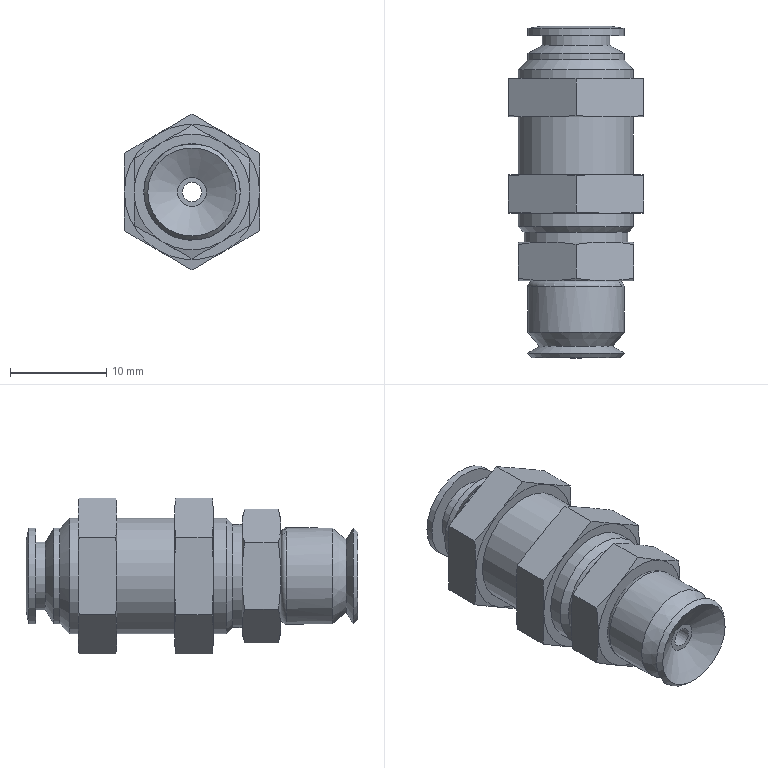Part | STEP file | 189171_ESG_10_SN_HA_QS_2_14b | 4 solids | 94 faces | box 14 x 34.4 x 16.166 mm | volume 3340 mm3 | cone 51 | plane 30 | cylinder 12 | torus 1 | commonest cylinder face diameters 10 x3 10.106 x2 2 x1 3.242 x1 4 x1 6 x1